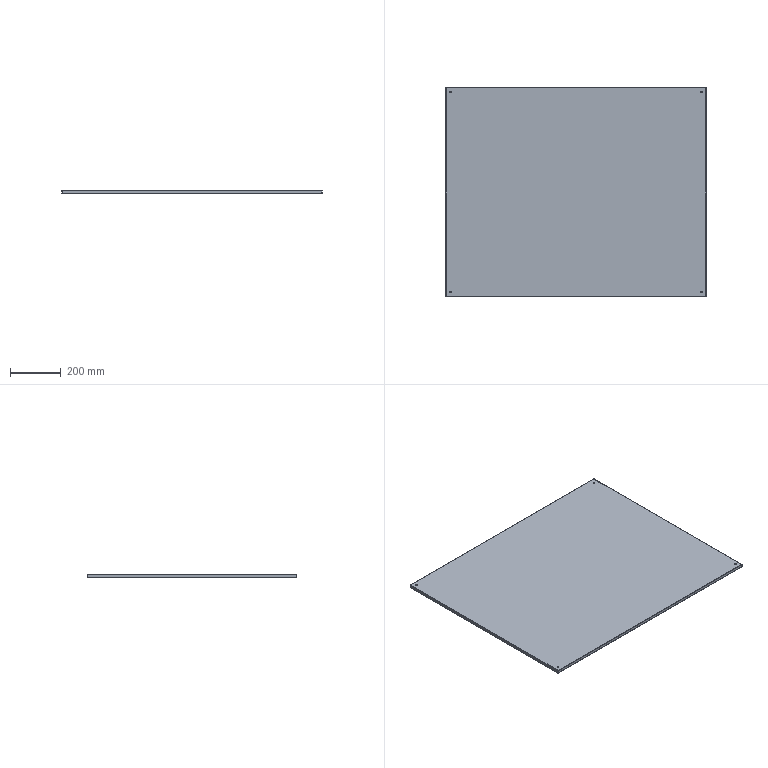Part | SolidWorks | features EdgeFlange 2, FlatPattern 1, ICE 1, SMBaseFlange 1, SheetMetal 1 | 1 solid | 78 faces | box 1027 x 827 x 13 mm | volume 1380132 mm3 | plane 38 | cylinder 24 | spline 16 | commonest cylinder face diameters 0.2 x8 3.2 x8 7 x8